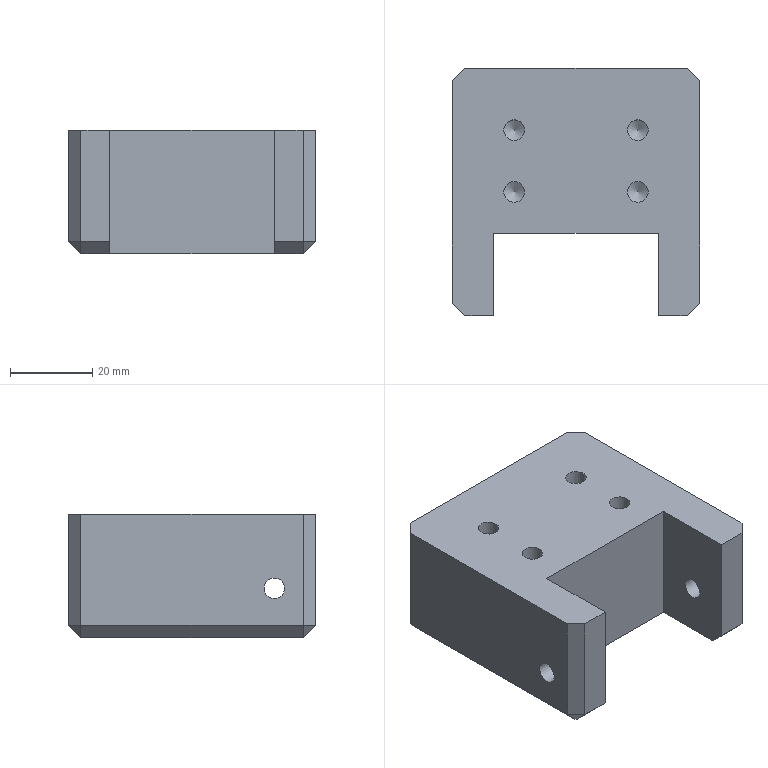Part | NX | features 5003_206_Bracket 2 | 1 solid | 33 faces | box 60 x 60 x 30 mm | volume 81572 mm3 | plane 23 | cylinder 6 | cone 4 | commonest cylinder face diameters 5 x6
STEP:
#1=CARTESIAN_POINT('',(18.525,-182.,-202.));
#2=VERTEX_POINT('',#1);
#3=CARTESIAN_POINT('',(25.525,-182.,-202.));
#4=VERTEX_POINT('',#3);
#5=CARTESIAN_POINT('',(28.525,-182.,-202.));
#6=DIRECTION('',(1.,0.,0.));
#7=VECTOR('',#6,1000.);
#8=LINE('',#5,#7);
#9=EDGE_CURVE('',#2,#4,#8,.T.);
#10=ORIENTED_EDGE('',*,*,#9,.F.);
#11=CARTESIAN_POINT('',(18.525,-182.,-229.));
#12=VERTEX_POINT('',#11);
#13=CARTESIAN_POINT('',(18.525,-182.,-201.999));
#14=DIRECTION('',(0.,0.,-1.));
#15=VECTOR('',#14,1000.);
#16=LINE('',#13,#15);
#17=EDGE_CURVE('',#2,#12,#16,.T.);
#18=ORIENTED_EDGE('',*,*,#17,.T.);
#19=CARTESIAN_POINT('',(25.525,-182.,-229.));
#20=VERTEX_POINT('',#19);
#21=CARTESIAN_POINT('',(28.525,-182.,-229.));
#22=DIRECTION('',(1.,0.,0.));
#23=VECTOR('',#22,1000.);
#24=LINE('',#21,#23);
#25=EDGE_CURVE('',#12,#20,#24,.T.);
#26=ORIENTED_EDGE('',*,*,#25,.T.);
#27=CARTESIAN_POINT('',(25.525,-182.,-202.));
#28=DIRECTION('',(0.,0.,1.));
#29=VECTOR('',#28,1000.);
#30=LINE('',#27,#29);
#31=EDGE_CURVE('',#20,#4,#30,.T.);
#32=ORIENTED_EDGE('',*,*,#31,.T.);
#33=EDGE_LOOP('',(#10,#18,#26,#32));
#34=FACE_BOUND('',#33,.T.);
#35=CARTESIAN_POINT('',(28.525,-182.,-202.));
#36=DIRECTION('',(0.,1.,0.));
#37=DIRECTION('',(-1.,0.,0.));
#38=AXIS2_PLACEMENT_3D('',#35,#36,#37);
#39=PLANE('',#38);
#40=ADVANCED_FACE('',(#34),#39,.F.);
#41=CARTESIAN_POINT('',(18.525,-169.5,-220.));
#42=VERTEX_POINT('',#41);
#43=CARTESIAN_POINT('',(18.525,-172.,-220.));
#44=DIRECTION('',(1.,0.,0.));
#45=DIRECTION('',(0.,1.,0.));
#46=AXIS2_PLACEMENT_3D('',#43,#44,#45);
#47=CIRCLE('',#46,2.5);
#48=EDGE_CURVE('',#42,#42,#47,.T.);
#49=ORIENTED_EDGE('',*,*,#48,.F.);
#50=EDGE_LOOP('',(#49));
#51=FACE_BOUND('',#50,.T.);
#52=CARTESIAN_POINT('',(28.525,-169.5,-220.));
#53=VERTEX_POINT('',#52);
#54=CARTESIAN_POINT('',(28.525,-172.,-220.));
#55=DIRECTION('',(1.,0.,0.));
#56=DIRECTION('',(0.,1.,0.));
#57=AXIS2_PLACEMENT_3D('',#54,#55,#56);
#58=CIRCLE('',#57,2.5);
#59=EDGE_CURVE('',#53,#53,#58,.T.);
#60=ORIENTED_EDGE('',*,*,#59,.T.);
#61=EDGE_LOOP('',(#60));
#62=FACE_BOUND('',#61,.T.);
#63=CARTESIAN_POINT('',(28.525,-172.,-220.));
#64=DIRECTION('',(1.,0.,0.));
#65=DIRECTION('',(0.,1.,0.));
#66=AXIS2_PLACEMENT_3D('',#63,#64,#65);
#67=CYLINDRICAL_SURFACE('',#66,2.5);
#68=ADVANCED_FACE('',(#51,#62),#67,.F.);
#69=CARTESIAN_POINT('',(18.525,-179.,-232.));
#70=VERTEX_POINT('',#69);
#71=CARTESIAN_POINT('',(18.525,-185.5,-225.5));
#72=DIRECTION('',(0.,-0.7071,0.7071));
#73=VECTOR('',#72,1000.);
#74=LINE('',#71,#73);
#75=EDGE_CURVE('',#12,#70,#74,.F.);
#76=ORIENTED_EDGE('',*,*,#75,.T.);
#77=CARTESIAN_POINT('',(25.525,-179.,-232.));
#78=VERTEX_POINT('',#77);
#79=CARTESIAN_POINT('',(28.525,-179.,-232.));
#80=DIRECTION('',(-1.,0.,0.));
#81=VECTOR('',#80,1000.);
#82=LINE('',#79,#81);
#83=EDGE_CURVE('',#78,#70,#82,.T.);
#84=ORIENTED_EDGE('',*,*,#83,.F.);
#85=CARTESIAN_POINT('',(25.525,-182.,-229.));
#86=DIRECTION('',(0.,-0.7071,0.7071));
#87=VECTOR('',#86,1000.);
#88=LINE('',#85,#87);
#89=EDGE_CURVE('',#20,#78,#88,.F.);
#90=ORIENTED_EDGE('',*,*,#89,.F.);
#91=ORIENTED_EDGE('',*,*,#25,.F.);
#92=EDGE_LOOP('',(#76,#84,#90,#91));
#93=FACE_BOUND('',#92,.T.);
#94=CARTESIAN_POINT('',(28.525,-182.,-229.));
#95=DIRECTION('',(0.,0.7071,0.7071));
#96=DIRECTION('',(1.,0.,0.));
#97=AXIS2_PLACEMENT_3D('',#94,#95,#96);
#98=PLANE('',#97);
#99=ADVANCED_FACE('',(#93),#98,.F.);
#100=ORIENTED_EDGE('',*,*,#59,.F.);
#101=EDGE_LOOP('',(#100));
#102=FACE_BOUND('',#101,.T.);
#103=CARTESIAN_POINT('',(28.525,-179.,-202.));
#104=VERTEX_POINT('',#103);
#105=CARTESIAN_POINT('',(28.525,-125.,-202.));
#106=VERTEX_POINT('',#105);
#107=CARTESIAN_POINT('',(28.525,-182.,-202.));
#108=DIRECTION('',(0.,1.,0.));
#109=VECTOR('',#108,1000.);
#110=LINE('',#107,#109);
#111=EDGE_CURVE('',#104,#106,#110,.T.);
#112=ORIENTED_EDGE('',*,*,#111,.F.);
#113=CARTESIAN_POINT('',(28.525,-179.,-229.));
#114=VERTEX_POINT('',#113);
#115=CARTESIAN_POINT('',(28.525,-179.,-202.));
#116=DIRECTION('',(0.,0.,-1.));
#117=VECTOR('',#116,1000.);
#118=LINE('',#115,#117);
#119=EDGE_CURVE('',#104,#114,#118,.T.);
#120=ORIENTED_EDGE('',*,*,#119,.T.);
#121=CARTESIAN_POINT('',(28.525,-125.,-229.));
#122=VERTEX_POINT('',#121);
#123=CARTESIAN_POINT('',(28.525,-182.,-229.));
#124=DIRECTION('',(0.,1.,0.));
#125=VECTOR('',#124,1000.);
#126=LINE('',#123,#125);
#127=EDGE_CURVE('',#114,#122,#126,.T.);
#128=ORIENTED_EDGE('',*,*,#127,.T.);
#129=CARTESIAN_POINT('',(28.525,-125.,-202.));
#130=DIRECTION('',(0.,0.,1.));
#131=VECTOR('',#130,1000.);
#132=LINE('',#129,#131);
#133=EDGE_CURVE('',#122,#106,#132,.T.);
#134=ORIENTED_EDGE('',*,*,#133,.T.);
#135=EDGE_LOOP('',(#112,#120,#128,#134));
#136=FACE_BOUND('',#135,.T.);
#137=CARTESIAN_POINT('',(28.525,-182.,-202.));
#138=DIRECTION('',(-1.,0.,0.));
#139=DIRECTION('',(0.,-1.,0.));
#140=AXIS2_PLACEMENT_3D('',#137,#138,#139);
#141=PLANE('',#140);
#142=ADVANCED_FACE('',(#102,#136),#141,.F.);
#143=CARTESIAN_POINT('',(25.525,-122.,-229.));
#144=VERTEX_POINT('',#143);
#145=CARTESIAN_POINT('',(-28.475,-122.,-229.));
#146=VERTEX_POINT('',#145);
#147=CARTESIAN_POINT('',(28.525,-122.,-229.));
#148=DIRECTION('',(-1.,0.,0.));
#149=VECTOR('',#148,1000.);
#150=LINE('',#147,#149);
#151=EDGE_CURVE('',#144,#146,#150,.T.);
#152=ORIENTED_EDGE('',*,*,#151,.T.);
#153=CARTESIAN_POINT('',(-28.475,-122.,-202.));
#154=VERTEX_POINT('',#153);
#155=CARTESIAN_POINT('',(-28.475,-122.,-202.));
#156=DIRECTION('',(0.,0.,1.));
#157=VECTOR('',#156,1000.);
#158=LINE('',#155,#157);
#159=EDGE_CURVE('',#146,#154,#158,.T.);
#160=ORIENTED_EDGE('',*,*,#159,.T.);
#161=CARTESIAN_POINT('',(25.525,-122.,-202.));
#162=VERTEX_POINT('',#161);
#163=CARTESIAN_POINT('',(28.525,-122.,-202.));
#164=DIRECTION('',(-1.,0.,0.));
#165=VECTOR('',#164,1000.);
#166=LINE('',#163,#165);
#167=EDGE_CURVE('',#162,#154,#166,.T.);
#168=ORIENTED_EDGE('',*,*,#167,.F.);
#169=CARTESIAN_POINT('',(25.525,-122.,-202.));
#170=DIRECTION('',(0.,0.,-1.));
#171=VECTOR('',#170,1000.);
#172=LINE('',#169,#171);
#173=EDGE_CURVE('',#162,#144,#172,.T.);
#174=ORIENTED_EDGE('',*,*,#173,.T.);
#175=EDGE_LOOP('',(#152,#160,#168,#174));
#176=FACE_BOUND('',#175,.T.);
#177=CARTESIAN_POINT('',(28.525,-122.,-202.));
#178=DIRECTION('',(0.,-1.,0.));
#179=DIRECTION('',(1.,0.,0.));
#180=AXIS2_PLACEMENT_3D('',#177,#178,#179);
#181=PLANE('',#180);
#182=ADVANCED_FACE('',(#176),#181,.F.);
#183=CARTESIAN_POINT('',(-31.475,-169.5,-220.));
#184=VERTEX_POINT('',#183);
#185=CARTESIAN_POINT('',(-31.475,-172.,-220.));
#186=DIRECTION('',(1.,0.,0.));
#187=DIRECTION('',(0.,1.,0.));
#188=AXIS2_PLACEMENT_3D('',#185,#186,#187);
#189=CIRCLE('',#188,2.5);
#190=EDGE_CURVE('',#184,#184,#189,.T.);
#191=ORIENTED_EDGE('',*,*,#190,.T.);
#192=EDGE_LOOP('',(#191));
#193=FACE_BOUND('',#192,.T.);
#194=CARTESIAN_POINT('',(-31.475,-125.,-202.));
#195=VERTEX_POINT('',#194);
#196=CARTESIAN_POINT('',(-31.475,-179.,-202.));
#197=VERTEX_POINT('',#196);
#198=CARTESIAN_POINT('',(-31.475,-182.,-202.));
#199=DIRECTION('',(0.,-1.,0.));
#200=VECTOR('',#199,1000.);
#201=LINE('',#198,#200);
#202=EDGE_CURVE('',#195,#197,#201,.T.);
#203=ORIENTED_EDGE('',*,*,#202,.F.);
#204=CARTESIAN_POINT('',(-31.475,-125.,-229.));
#205=VERTEX_POINT('',#204);
#206=CARTESIAN_POINT('',(-31.475,-125.,-202.));
#207=DIRECTION('',(0.,0.,-1.));
#208=VECTOR('',#207,1000.);
#209=LINE('',#206,#208);
#210=EDGE_CURVE('',#195,#205,#209,.T.);
#211=ORIENTED_EDGE('',*,*,#210,.T.);
#212=CARTESIAN_POINT('',(-31.475,-179.,-229.));
#213=VERTEX_POINT('',#212);
#214=CARTESIAN_POINT('',(-31.475,-182.,-229.));
#215=DIRECTION('',(0.,-1.,0.));
#216=VECTOR('',#215,1000.);
#217=LINE('',#214,#216);
#218=EDGE_CURVE('',#205,#213,#217,.T.);
#219=ORIENTED_EDGE('',*,*,#218,.T.);
#220=CARTESIAN_POINT('',(-31.475,-179.,-202.));
#221=DIRECTION('',(0.,0.,1.));
#222=VECTOR('',#221,1000.);
#223=LINE('',#220,#222);
#224=EDGE_CURVE('',#213,#197,#223,.T.);
#225=ORIENTED_EDGE('',*,*,#224,.T.);
#226=EDGE_LOOP('',(#203,#211,#219,#225));
#227=FACE_BOUND('',#226,.T.);
#228=CARTESIAN_POINT('',(-31.475,-182.,-202.));
#229=DIRECTION('',(1.,0.,0.));
#230=DIRECTION('',(0.,1.,0.));
#231=AXIS2_PLACEMENT_3D('',#228,#229,#230);
#232=PLANE('',#231);
#233=ADVANCED_FACE('',(#193,#227),#232,.F.);
#234=CARTESIAN_POINT('',(-28.475,-182.,-229.));
#235=VERTEX_POINT('',#234);
#236=CARTESIAN_POINT('',(-21.475,-182.,-229.));
#237=VERTEX_POINT('',#236);
#238=CARTESIAN_POINT('',(28.525,-182.,-229.));
#239=DIRECTION('',(1.,0.,0.));
#240=VECTOR('',#239,1000.);
#241=LINE('',#238,#240);
#242=EDGE_CURVE('',#235,#237,#241,.T.);
#243=ORIENTED_EDGE('',*,*,#242,.T.);
#244=CARTESIAN_POINT('',(-21.475,-182.,-202.));
#245=VERTEX_POINT('',#244);
#246=CARTESIAN_POINT('',(-21.475,-182.,-201.999));
#247=DIRECTION('',(0.,0.,-1.));
#248=VECTOR('',#247,1000.);
#249=LINE('',#246,#248);
#250=EDGE_CURVE('',#245,#237,#249,.T.);
#251=ORIENTED_EDGE('',*,*,#250,.F.);
#252=CARTESIAN_POINT('',(-28.475,-182.,-202.));
#253=VERTEX_POINT('',#252);
#254=CARTESIAN_POINT('',(28.525,-182.,-202.));
#255=DIRECTION('',(1.,0.,0.));
#256=VECTOR('',#255,1000.);
#257=LINE('',#254,#256);
#258=EDGE_CURVE('',#253,#245,#257,.T.);
#259=ORIENTED_EDGE('',*,*,#258,.F.);
#260=CARTESIAN_POINT('',(-28.475,-182.,-202.));
#261=DIRECTION('',(0.,0.,-1.));
#262=VECTOR('',#261,1000.);
#263=LINE('',#260,#262);
#264=EDGE_CURVE('',#253,#235,#263,.T.);
#265=ORIENTED_EDGE('',*,*,#264,.T.);
#266=EDGE_LOOP('',(#243,#251,#259,#265));
#267=FACE_BOUND('',#266,.T.);
#268=CARTESIAN_POINT('',(28.525,-182.,-202.));
#269=DIRECTION('',(0.,1.,0.));
#270=DIRECTION('',(-1.,0.,0.));
#271=AXIS2_PLACEMENT_3D('',#268,#269,#270);
#272=PLANE('',#271);
#273=ADVANCED_FACE('',(#267),#272,.F.);
#274=CARTESIAN_POINT('',(18.525,-162.,-202.));
#275=VERTEX_POINT('',#274);
#276=CARTESIAN_POINT('',(18.525,-162.,-202.));
#277=DIRECTION('',(0.,-1.,0.));
#278=VECTOR('',#277,1000.);
#279=LINE('',#276,#278);
#280=EDGE_CURVE('',#275,#2,#279,.T.);
#281=ORIENTED_EDGE('',*,*,#280,.T.);
#282=ORIENTED_EDGE('',*,*,#9,.T.);
#283=CARTESIAN_POINT('',(27.025,-180.5,-202.));
#284=DIRECTION('',(-0.7071,-0.7071,0.));
#285=VECTOR('',#284,1000.);
#286=LINE('',#283,#285);
#287=EDGE_CURVE('',#4,#104,#286,.F.);
#288=ORIENTED_EDGE('',*,*,#287,.T.);
#289=ORIENTED_EDGE('',*,*,#111,.T.);
#290=CARTESIAN_POINT('',(57.025,-153.5,-202.));
#291=DIRECTION('',(0.7071,-0.7071,0.));
#292=VECTOR('',#291,1000.);
#293=LINE('',#290,#292);
#294=EDGE_CURVE('',#106,#162,#293,.F.);
#295=ORIENTED_EDGE('',*,*,#294,.T.);
#296=ORIENTED_EDGE('',*,*,#167,.T.);
#297=CARTESIAN_POINT('',(-29.975,-123.5,-202.));
#298=DIRECTION('',(0.7071,0.7071,0.));
#299=VECTOR('',#298,1000.);
#300=LINE('',#297,#299);
#301=EDGE_CURVE('',#154,#195,#300,.F.);
#302=ORIENTED_EDGE('',*,*,#301,.T.);
#303=ORIENTED_EDGE('',*,*,#202,.T.);
#304=CARTESIAN_POINT('',(0.025,-210.5,-202.));
#305=DIRECTION('',(-0.7071,0.7071,0.));
#306=VECTOR('',#305,1000.);
#307=LINE('',#304,#306);
#308=EDGE_CURVE('',#197,#253,#307,.F.);
#309=ORIENTED_EDGE('',*,*,#308,.T.);
#310=ORIENTED_EDGE('',*,*,#258,.T.);
#311=CARTESIAN_POINT('',(-21.475,-162.,-202.));
#312=VERTEX_POINT('',#311);
#313=CARTESIAN_POINT('',(-21.475,-162.,-202.));
#314=DIRECTION('',(0.,1.,0.));
#315=VECTOR('',#314,1000.);
#316=LINE('',#313,#315);
#317=EDGE_CURVE('',#245,#312,#316,.T.);
#318=ORIENTED_EDGE('',*,*,#317,.T.);
#319=CARTESIAN_POINT('',(18.525,-162.,-202.));
#320=DIRECTION('',(1.,0.,0.));
#321=VECTOR('',#320,1000.);
#322=LINE('',#319,#321);
#323=EDGE_CURVE('',#312,#275,#322,.T.);
#324=ORIENTED_EDGE('',*,*,#323,.T.);
#325=EDGE_LOOP('',(#281,#282,#288,#289,#295,#296,#302,#303,#309,#310,#318,#324));
#326=FACE_BOUND('',#325,.T.);
#327=CARTESIAN_POINT('',(-16.475,-149.5,-202.));
#328=VERTEX_POINT('',#327);
#329=CARTESIAN_POINT('',(-16.475,-152.,-202.));
#330=DIRECTION('',(0.,0.,1.));
#331=DIRECTION('',(0.,1.,0.));
#332=AXIS2_PLACEMENT_3D('',#329,#330,#331);
#333=CIRCLE('',#332,2.5);
#334=EDGE_CURVE('',#328,#328,#333,.T.);
#335=ORIENTED_EDGE('',*,*,#334,.F.);
#336=EDGE_LOOP('',(#335));
#337=FACE_BOUND('',#336,.T.);
#338=CARTESIAN_POINT('',(13.525,-134.5,-202.));
#339=VERTEX_POINT('',#338);
#340=CARTESIAN_POINT('',(13.525,-137.,-202.));
#341=DIRECTION('',(0.,0.,1.));
#342=DIRECTION('',(0.,1.,0.));
#343=AXIS2_PLACEMENT_3D('',#340,#341,#342);
#344=CIRCLE('',#343,2.5);
#345=EDGE_CURVE('',#339,#339,#344,.T.);
#346=ORIENTED_EDGE('',*,*,#345,.F.);
#347=EDGE_LOOP('',(#346));
#348=FACE_BOUND('',#347,.T.);
#349=CARTESIAN_POINT('',(-16.475,-134.5,-202.));
#350=VERTEX_POINT('',#349);
#351=CARTESIAN_POINT('',(-16.475,-137.,-202.));
#352=DIRECTION('',(0.,0.,1.));
#353=DIRECTION('',(0.,1.,0.));
#354=AXIS2_PLACEMENT_3D('',#351,#352,#353);
#355=CIRCLE('',#354,2.5);
#356=EDGE_CURVE('',#350,#350,#355,.T.);
#357=ORIENTED_EDGE('',*,*,#356,.F.);
#358=EDGE_LOOP('',(#357));
#359=FACE_BOUND('',#358,.T.);
#360=CARTESIAN_POINT('',(13.525,-149.5,-202.));
#361=VERTEX_POINT('',#360);
#362=CARTESIAN_POINT('',(13.525,-152.,-202.));
#363=DIRECTION('',(0.,0.,1.));
#364=DIRECTION('',(0.,1.,0.));
#365=AXIS2_PLACEMENT_3D('',#362,#363,#364);
#366=CIRCLE('',#365,2.5);
#367=EDGE_CURVE('',#361,#361,#366,.T.);
#368=ORIENTED_EDGE('',*,*,#367,.F.);
#369=EDGE_LOOP('',(#368));
#370=FACE_BOUND('',#369,.T.);
#371=CARTESIAN_POINT('',(28.525,-182.,-202.));
#372=DIRECTION('',(0.,0.,1.));
#373=DIRECTION('',(0.,1.,0.));
#374=AXIS2_PLACEMENT_3D('',#371,#372,#373);
#375=PLANE('',#374);
#376=ADVANCED_FACE('',(#326,#337,#348,#359,#370),#375,.T.);
#377=ORIENTED_EDGE('',*,*,#83,.T.);
#378=CARTESIAN_POINT('',(18.525,-162.,-232.));
#379=VERTEX_POINT('',#378);
#380=CARTESIAN_POINT('',(18.525,-162.,-232.));
#381=DIRECTION('',(0.,-1.,0.));
#382=VECTOR('',#381,1000.);
#383=LINE('',#380,#382);
#384=EDGE_CURVE('',#379,#70,#383,.T.);
#385=ORIENTED_EDGE('',*,*,#384,.F.);
#386=CARTESIAN_POINT('',(-21.475,-162.,-232.));
#387=VERTEX_POINT('',#386);
#388=CARTESIAN_POINT('',(18.525,-162.,-232.));
#389=DIRECTION('',(1.,0.,0.));
#390=VECTOR('',#389,1000.);
#391=LINE('',#388,#390);
#392=EDGE_CURVE('',#387,#379,#391,.T.);
#393=ORIENTED_EDGE('',*,*,#392,.F.);
#394=CARTESIAN_POINT('',(-21.475,-179.,-232.));
#395=VERTEX_POINT('',#394);
#396=CARTESIAN_POINT('',(-21.475,-162.,-232.));
#397=DIRECTION('',(0.,1.,0.));
#398=VECTOR('',#397,1000.);
#399=LINE('',#396,#398);
#400=EDGE_CURVE('',#395,#387,#399,.T.);
#401=ORIENTED_EDGE('',*,*,#400,.F.);
#402=CARTESIAN_POINT('',(-28.475,-179.,-232.));
#403=VERTEX_POINT('',#402);
#404=CARTESIAN_POINT('',(28.525,-179.,-232.));
#405=DIRECTION('',(-1.,0.,0.));
#406=VECTOR('',#405,1000.);
#407=LINE('',#404,#406);
#408=EDGE_CURVE('',#395,#403,#407,.T.);
#409=ORIENTED_EDGE('',*,*,#408,.T.);
#410=CARTESIAN_POINT('',(-28.475,-125.,-232.));
#411=VERTEX_POINT('',#410);
#412=CARTESIAN_POINT('',(-28.475,-182.,-232.));
#413=DIRECTION('',(0.,1.,0.));
#414=VECTOR('',#413,1000.);
#415=LINE('',#412,#414);
#416=EDGE_CURVE('',#403,#411,#415,.T.);
#417=ORIENTED_EDGE('',*,*,#416,.T.);
#418=CARTESIAN_POINT('',(25.525,-125.,-232.));
#419=VERTEX_POINT('',#418);
#420=CARTESIAN_POINT('',(28.525,-125.,-232.));
#421=DIRECTION('',(1.,0.,0.));
#422=VECTOR('',#421,1000.);
#423=LINE('',#420,#422);
#424=EDGE_CURVE('',#411,#419,#423,.T.);
#425=ORIENTED_EDGE('',*,*,#424,.T.);
#426=CARTESIAN_POINT('',(25.525,-182.,-232.));
#427=DIRECTION('',(0.,-1.,0.));
#428=VECTOR('',#427,1000.);
#429=LINE('',#426,#428);
#430=EDGE_CURVE('',#419,#78,#429,.T.);
#431=ORIENTED_EDGE('',*,*,#430,.T.);
#432=EDGE_LOOP('',(#377,#385,#393,#401,#409,#417,#425,#431));
#433=FACE_BOUND('',#432,.T.);
#434=CARTESIAN_POINT('',(28.525,-182.,-232.));
#435=DIRECTION('',(0.,0.,1.));
#436=DIRECTION('',(0.,1.,0.));
#437=AXIS2_PLACEMENT_3D('',#434,#435,#436);
#438=PLANE('',#437);
#439=ADVANCED_FACE('',(#433),#438,.F.);
#440=CARTESIAN_POINT('',(-21.475,-174.5,-220.));
#441=VERTEX_POINT('',#440);
#442=CARTESIAN_POINT('',(-21.475,-172.,-220.));
#443=DIRECTION('',(-1.,0.,0.));
#444=DIRECTION('',(0.,-1.,0.));
#445=AXIS2_PLACEMENT_3D('',#442,#443,#444);
#446=CIRCLE('',#445,2.5);
#447=EDGE_CURVE('',#441,#441,#446,.T.);
#448=ORIENTED_EDGE('',*,*,#447,.F.);
#449=EDGE_LOOP('',(#448));
#450=FACE_BOUND('',#449,.T.);
#451=ORIENTED_EDGE('',*,*,#190,.F.);
#452=EDGE_LOOP('',(#451));
#453=FACE_BOUND('',#452,.T.);
#454=CARTESIAN_POINT('',(28.525,-172.,-220.));
#455=DIRECTION('',(1.,0.,0.));
#456=DIRECTION('',(0.,1.,0.));
#457=AXIS2_PLACEMENT_3D('',#454,#455,#456);
#458=CYLINDRICAL_SURFACE('',#457,2.5);
#459=ADVANCED_FACE('',(#450,#453),#458,.F.);
#460=CARTESIAN_POINT('',(13.525,-152.,-211.502));
#461=VERTEX_POINT('',#460);
#462=VERTEX_LOOP('',#461);
#463=FACE_BOUND('',#462,.T.);
#464=CARTESIAN_POINT('',(13.525,-149.5,-210.));
#465=VERTEX_POINT('',#464);
#466=CARTESIAN_POINT('',(13.525,-152.,-210.));
#467=DIRECTION('',(0.,0.,1.));
#468=DIRECTION('',(0.,1.,0.));
#469=AXIS2_PLACEMENT_3D('',#466,#467,#468);
#470=CIRCLE('',#469,2.5);
#471=EDGE_CURVE('',#465,#465,#470,.T.);
#472=ORIENTED_EDGE('',*,*,#471,.T.);
#473=EDGE_LOOP('',(#472));
#474=FACE_BOUND('',#473,.T.);
#475=CARTESIAN_POINT('',(13.525,-152.,-210.));
#476=DIRECTION('',(0.,0.,1.));
#477=DIRECTION('',(0.,1.,0.));
#478=AXIS2_PLACEMENT_3D('',#475,#476,#477);
#479=CONICAL_SURFACE('',#478,2.5,1.03);
#480=ADVANCED_FACE('',(#463,#474),#479,.F.);
#481=ORIENTED_EDGE('',*,*,#471,.F.);
#482=EDGE_LOOP('',(#481));
#483=FACE_BOUND('',#482,.T.);
#484=ORIENTED_EDGE('',*,*,#367,.T.);
#485=EDGE_LOOP('',(#484));
#486=FACE_BOUND('',#485,.T.);
#487=CARTESIAN_POINT('',(13.525,-152.,-202.));
#488=DIRECTION('',(0.,0.,1.));
#489=DIRECTION('',(0.,1.,0.));
#490=AXIS2_PLACEMENT_3D('',#487,#488,#489);
#491=CYLINDRICAL_SURFACE('',#490,2.5);
#492=ADVANCED_FACE('',(#483,#486),#491,.F.);
#493=CARTESIAN_POINT('',(-16.475,-137.,-211.502));
#494=VERTEX_POINT('',#493);
#495=VERTEX_LOOP('',#494);
#496=FACE_BOUND('',#495,.T.);
#497=CARTESIAN_POINT('',(-16.475,-134.5,-210.));
#498=VERTEX_POINT('',#497);
#499=CARTESIAN_POINT('',(-16.475,-137.,-210.));
#500=DIRECTION('',(0.,0.,1.));
#501=DIRECTION('',(0.,1.,0.));
#502=AXIS2_PLACEMENT_3D('',#499,#500,#501);
#503=CIRCLE('',#502,2.5);
#504=EDGE_CURVE('',#498,#498,#503,.T.);
#505=ORIENTED_EDGE('',*,*,#504,.T.);
#506=EDGE_LOOP('',(#505));
#507=FACE_BOUND('',#506,.T.);
#508=CARTESIAN_POINT('',(-16.475,-137.,-210.));
#509=DIRECTION('',(0.,0.,1.));
#510=DIRECTION('',(0.,1.,0.));
#511=AXIS2_PLACEMENT_3D('',#508,#509,#510);
#512=CONICAL_SURFACE('',#511,2.5,1.03);
#513=ADVANCED_FACE('',(#496,#507),#512,.F.);
#514=ORIENTED_EDGE('',*,*,#504,.F.);
#515=EDGE_LOOP('',(#514));
#516=FACE_BOUND('',#515,.T.);
#517=ORIENTED_EDGE('',*,*,#356,.T.);
#518=EDGE_LOOP('',(#517));
#519=FACE_BOUND('',#518,.T.);
#520=CARTESIAN_POINT('',(-16.475,-137.,-202.));
#521=DIRECTION('',(0.,0.,1.));
#522=DIRECTION('',(0.,1.,0.));
#523=AXIS2_PLACEMENT_3D('',#520,#521,#522);
#524=CYLINDRICAL_SURFACE('',#523,2.5);
#525=ADVANCED_FACE('',(#516,#519),#524,.F.);
#526=CARTESIAN_POINT('',(13.525,-137.,-211.502));
#527=VERTEX_POINT('',#526);
#528=VERTEX_LOOP('',#527);
#529=FACE_BOUND('',#528,.T.);
#530=CARTESIAN_POINT('',(13.525,-134.5,-210.));
#531=VERTEX_POINT('',#530);
#532=CARTESIAN_POINT('',(13.525,-137.,-210.));
#533=DIRECTION('',(0.,0.,1.));
#534=DIRECTION('',(0.,1.,0.));
#535=AXIS2_PLACEMENT_3D('',#532,#533,#534);
#536=CIRCLE('',#535,2.5);
#537=EDGE_CURVE('',#531,#531,#536,.T.);
#538=ORIENTED_EDGE('',*,*,#537,.T.);
#539=EDGE_LOOP('',(#538));
#540=FACE_BOUND('',#539,.T.);
#541=CARTESIAN_POINT('',(13.525,-137.,-210.));
#542=DIRECTION('',(0.,0.,1.));
#543=DIRECTION('',(0.,1.,0.));
#544=AXIS2_PLACEMENT_3D('',#541,#542,#543);
#545=CONICAL_SURFACE('',#544,2.5,1.03);
#546=ADVANCED_FACE('',(#529,#540),#545,.F.);
#547=ORIENTED_EDGE('',*,*,#537,.F.);
#548=EDGE_LOOP('',(#547));
#549=FACE_BOUND('',#548,.T.);
#550=ORIENTED_EDGE('',*,*,#345,.T.);
#551=EDGE_LOOP('',(#550));
#552=FACE_BOUND('',#551,.T.);
#553=CARTESIAN_POINT('',(13.525,-137.,-202.));
#554=DIRECTION('',(0.,0.,1.));
#555=DIRECTION('',(0.,1.,0.));
#556=AXIS2_PLACEMENT_3D('',#553,#554,#555);
#557=CYLINDRICAL_SURFACE('',#556,2.5);
#558=ADVANCED_FACE('',(#549,#552),#557,.F.);
#559=CARTESIAN_POINT('',(-16.475,-152.,-211.502));
#560=VERTEX_POINT('',#559);
#561=VERTEX_LOOP('',#560);
#562=FACE_BOUND('',#561,.T.);
#563=CARTESIAN_POINT('',(-16.475,-149.5,-210.));
#564=VERTEX_POINT('',#563);
#565=CARTESIAN_POINT('',(-16.475,-152.,-210.));
#566=DIRECTION('',(0.,0.,1.));
#567=DIRECTION('',(0.,1.,0.));
#568=AXIS2_PLACEMENT_3D('',#565,#566,#567);
#569=CIRCLE('',#568,2.5);
#570=EDGE_CURVE('',#564,#564,#569,.T.);
#571=ORIENTED_EDGE('',*,*,#570,.T.);
#572=EDGE_LOOP('',(#571));
#573=FACE_BOUND('',#572,.T.);
#574=CARTESIAN_POINT('',(-16.475,-152.,-210.));
#575=DIRECTION('',(0.,0.,1.));
#576=DIRECTION('',(0.,1.,0.));
#577=AXIS2_PLACEMENT_3D('',#574,#575,#576);
#578=CONICAL_SURFACE('',#577,2.5,1.03);
#579=ADVANCED_FACE('',(#562,#573),#578,.F.);
#580=ORIENTED_EDGE('',*,*,#570,.F.);
#581=EDGE_LOOP('',(#580));
#582=FACE_BOUND('',#581,.T.);
#583=ORIENTED_EDGE('',*,*,#334,.T.);
#584=EDGE_LOOP('',(#583));
#585=FACE_BOUND('',#584,.T.);
#586=CARTESIAN_POINT('',(-16.475,-152.,-202.));
#587=DIRECTION('',(0.,0.,1.));
#588=DIRECTION('',(0.,1.,0.));
#589=AXIS2_PLACEMENT_3D('',#586,#587,#588);
#590=CYLINDRICAL_SURFACE('',#589,2.5);
#591=ADVANCED_FACE('',(#582,#585),#590,.F.);
#592=ORIENTED_EDGE('',*,*,#287,.F.);
#593=ORIENTED_EDGE('',*,*,#31,.F.);
#594=CARTESIAN_POINT('',(25.525,-182.,-229.));
#595=DIRECTION('',(0.7071,0.7071,0.));
#596=VECTOR('',#595,1000.);
#597=LINE('',#594,#596);
#598=EDGE_CURVE('',#114,#20,#597,.F.);
#599=ORIENTED_EDGE('',*,*,#598,.F.);
#600=ORIENTED_EDGE('',*,*,#119,.F.);
#601=EDGE_LOOP('',(#592,#593,#599,#600));
#602=FACE_BOUND('',#601,.T.);
#603=CARTESIAN_POINT('',(28.525,-179.,-202.));
#604=DIRECTION('',(-0.7071,0.7071,0.));
#605=DIRECTION('',(0.,0.,-1.));
#606=AXIS2_PLACEMENT_3D('',#603,#604,#605);
#607=PLANE('',#606);
#608=ADVANCED_FACE('',(#602),#607,.F.);
#609=ORIENTED_EDGE('',*,*,#308,.F.);
#610=ORIENTED_EDGE('',*,*,#224,.F.);
#611=CARTESIAN_POINT('',(-31.475,-179.,-229.));
#612=DIRECTION('',(0.7071,-0.7071,0.));
#613=VECTOR('',#612,1000.);
#614=LINE('',#611,#613);
#615=EDGE_CURVE('',#235,#213,#614,.F.);
#616=ORIENTED_EDGE('',*,*,#615,.F.);
#617=ORIENTED_EDGE('',*,*,#264,.F.);
#618=EDGE_LOOP('',(#609,#610,#616,#617));
#619=FACE_BOUND('',#618,.T.);
#620=CARTESIAN_POINT('',(-28.475,-182.,-202.));
#621=DIRECTION('',(0.7071,0.7071,0.));
#622=DIRECTION('',(0.,0.,-1.));
#623=AXIS2_PLACEMENT_3D('',#620,#621,#622);
#624=PLANE('',#623);
#625=ADVANCED_FACE('',(#619),#624,.F.);
#626=CARTESIAN_POINT('',(-21.475,-185.5,-225.5));
#627=DIRECTION('',(0.,0.7071,-0.7071));
#628=VECTOR('',#627,1000.);
#629=LINE('',#626,#628);
#630=EDGE_CURVE('',#395,#237,#629,.F.);
#631=ORIENTED_EDGE('',*,*,#630,.T.);
#632=ORIENTED_EDGE('',*,*,#242,.F.);
#633=CARTESIAN_POINT('',(-28.475,-180.5,-230.5));
#634=DIRECTION('',(0.,0.7071,-0.7071));
#635=VECTOR('',#634,1000.);
#636=LINE('',#633,#635);
#637=EDGE_CURVE('',#403,#235,#636,.F.);
#638=ORIENTED_EDGE('',*,*,#637,.F.);
#639=ORIENTED_EDGE('',*,*,#408,.F.);
#640=EDGE_LOOP('',(#631,#632,#638,#639));
#641=FACE_BOUND('',#640,.T.);
#642=CARTESIAN_POINT('',(28.525,-182.,-229.));
#643=DIRECTION('',(0.,0.7071,0.7071));
#644=DIRECTION('',(1.,0.,0.));
#645=AXIS2_PLACEMENT_3D('',#642,#643,#644);
#646=PLANE('',#645);
#647=ADVANCED_FACE('',(#641),#646,.F.);
#648=ORIENTED_EDGE('',*,*,#598,.T.);
#649=ORIENTED_EDGE('',*,*,#89,.T.);
#650=CARTESIAN_POINT('',(27.025,-179.,-230.5));
#651=DIRECTION('',(-0.7071,0.,-0.7071));
#652=VECTOR('',#651,1000.);
#653=LINE('',#650,#652);
#654=EDGE_CURVE('',#114,#78,#653,.T.);
#655=ORIENTED_EDGE('',*,*,#654,.F.);
#656=EDGE_LOOP('',(#648,#649,#655));
#657=FACE_BOUND('',#656,.T.);
#658=CARTESIAN_POINT('',(25.525,-182.,-229.));
#659=DIRECTION('',(0.5774,-0.5774,-0.5774));
#660=DIRECTION('',(-0.7071,0.,-0.7071));
#661=AXIS2_PLACEMENT_3D('',#658,#659,#660);
#662=PLANE('',#661);
#663=ADVANCED_FACE('',(#657),#662,.T.);
#664=ORIENTED_EDGE('',*,*,#637,.T.);
#665=ORIENTED_EDGE('',*,*,#615,.T.);
#666=CARTESIAN_POINT('',(-31.475,-179.,-229.));
#667=DIRECTION('',(-0.7071,0.,0.7071));
#668=VECTOR('',#667,1000.);
#669=LINE('',#666,#668);
#670=EDGE_CURVE('',#403,#213,#669,.T.);
#671=ORIENTED_EDGE('',*,*,#670,.F.);
#672=EDGE_LOOP('',(#664,#665,#671));
#673=FACE_BOUND('',#672,.T.);
#674=CARTESIAN_POINT('',(-31.475,-179.,-229.));
#675=DIRECTION('',(-0.5774,-0.5774,-0.5774));
#676=DIRECTION('',(-0.7071,0.,0.7071));
#677=AXIS2_PLACEMENT_3D('',#674,#675,#676);
#678=PLANE('',#677);
#679=ADVANCED_FACE('',(#673),#678,.T.);
#680=ORIENTED_EDGE('',*,*,#654,.T.);
#681=ORIENTED_EDGE('',*,*,#430,.F.);
#682=CARTESIAN_POINT('',(25.525,-125.,-232.));
#683=DIRECTION('',(0.7071,0.,0.7071));
#684=VECTOR('',#683,1000.);
#685=LINE('',#682,#684);
#686=EDGE_CURVE('',#122,#419,#685,.F.);
#687=ORIENTED_EDGE('',*,*,#686,.F.);
#688=ORIENTED_EDGE('',*,*,#127,.F.);
#689=EDGE_LOOP('',(#680,#681,#687,#688));
#690=FACE_BOUND('',#689,.T.);
#691=CARTESIAN_POINT('',(28.525,-182.,-229.));
#692=DIRECTION('',(-0.7071,0.,0.7071));
#693=DIRECTION('',(0.,1.,0.));
#694=AXIS2_PLACEMENT_3D('',#691,#692,#693);
#695=PLANE('',#694);
#696=ADVANCED_FACE('',(#690),#695,.F.);
#697=ORIENTED_EDGE('',*,*,#294,.F.);
#698=ORIENTED_EDGE('',*,*,#133,.F.);
#699=CARTESIAN_POINT('',(27.025,-123.5,-229.));
#700=DIRECTION('',(-0.7071,0.7071,0.));
#701=VECTOR('',#700,1000.);
#702=LINE('',#699,#701);
#703=EDGE_CURVE('',#144,#122,#702,.F.);
#704=ORIENTED_EDGE('',*,*,#703,.F.);
#705=ORIENTED_EDGE('',*,*,#173,.F.);
#706=EDGE_LOOP('',(#697,#698,#704,#705));
#707=FACE_BOUND('',#706,.T.);
#708=CARTESIAN_POINT('',(25.525,-122.,-202.));
#709=DIRECTION('',(-0.7071,-0.7071,0.));
#710=DIRECTION('',(0.,0.,-1.));
#711=AXIS2_PLACEMENT_3D('',#708,#709,#710);
#712=PLANE('',#711);
#713=ADVANCED_FACE('',(#707),#712,.F.);
#714=ORIENTED_EDGE('',*,*,#301,.F.);
#715=ORIENTED_EDGE('',*,*,#159,.F.);
#716=CARTESIAN_POINT('',(-28.475,-122.,-229.));
#717=DIRECTION('',(-0.7071,-0.7071,0.));
#718=VECTOR('',#717,1000.);
#719=LINE('',#716,#718);
#720=EDGE_CURVE('',#205,#146,#719,.F.);
#721=ORIENTED_EDGE('',*,*,#720,.F.);
#722=ORIENTED_EDGE('',*,*,#210,.F.);
#723=EDGE_LOOP('',(#714,#715,#721,#722));
#724=FACE_BOUND('',#723,.T.);
#725=CARTESIAN_POINT('',(-31.475,-125.,-202.));
#726=DIRECTION('',(0.7071,-0.7071,0.));
#727=DIRECTION('',(0.,0.,-1.));
#728=AXIS2_PLACEMENT_3D('',#725,#726,#727);
#729=PLANE('',#728);
#730=ADVANCED_FACE('',(#724),#729,.F.);
#731=ORIENTED_EDGE('',*,*,#670,.T.);
#732=ORIENTED_EDGE('',*,*,#218,.F.);
#733=CARTESIAN_POINT('',(-29.975,-125.,-230.5));
#734=DIRECTION('',(0.7071,0.,-0.7071));
#735=VECTOR('',#734,1000.);
#736=LINE('',#733,#735);
#737=EDGE_CURVE('',#411,#205,#736,.F.);
#738=ORIENTED_EDGE('',*,*,#737,.F.);
#739=ORIENTED_EDGE('',*,*,#416,.F.);
#740=EDGE_LOOP('',(#731,#732,#738,#739));
#741=FACE_BOUND('',#740,.T.);
#742=CARTESIAN_POINT('',(-31.475,-182.,-229.));
#743=DIRECTION('',(0.7071,0.,0.7071));
#744=DIRECTION('',(0.,-1.,0.));
#745=AXIS2_PLACEMENT_3D('',#742,#743,#744);
#746=PLANE('',#745);
#747=ADVANCED_FACE('',(#741),#746,.F.);
#748=ORIENTED_EDGE('',*,*,#703,.T.);
#749=ORIENTED_EDGE('',*,*,#686,.T.);
#750=CARTESIAN_POINT('',(25.525,-125.,-232.));
#751=DIRECTION('',(0.,-0.7071,-0.7071));
#752=VECTOR('',#751,1000.);
#753=LINE('',#750,#752);
#754=EDGE_CURVE('',#144,#419,#753,.T.);
#755=ORIENTED_EDGE('',*,*,#754,.F.);
#756=EDGE_LOOP('',(#748,#749,#755));
#757=FACE_BOUND('',#756,.T.);
#758=CARTESIAN_POINT('',(25.525,-125.,-232.));
#759=DIRECTION('',(0.5774,0.5774,-0.5774));
#760=DIRECTION('',(-0.7071,0.,-0.7071));
#761=AXIS2_PLACEMENT_3D('',#758,#759,#760);
#762=PLANE('',#761);
#763=ADVANCED_FACE('',(#757),#762,.T.);
#764=ORIENTED_EDGE('',*,*,#737,.T.);
#765=ORIENTED_EDGE('',*,*,#720,.T.);
#766=CARTESIAN_POINT('',(-28.475,-122.,-229.));
#767=DIRECTION('',(0.,0.7071,0.7071));
#768=VECTOR('',#767,1000.);
#769=LINE('',#766,#768);
#770=EDGE_CURVE('',#411,#146,#769,.T.);
#771=ORIENTED_EDGE('',*,*,#770,.F.);
#772=EDGE_LOOP('',(#764,#765,#771));
#773=FACE_BOUND('',#772,.T.);
#774=CARTESIAN_POINT('',(-28.475,-122.,-229.));
#775=DIRECTION('',(-0.5774,0.5774,-0.5774));
#776=DIRECTION('',(-0.7071,0.,0.7071));
#777=AXIS2_PLACEMENT_3D('',#774,#775,#776);
#778=PLANE('',#777);
#779=ADVANCED_FACE('',(#773),#778,.T.);
#780=ORIENTED_EDGE('',*,*,#754,.T.);
#781=ORIENTED_EDGE('',*,*,#424,.F.);
#782=ORIENTED_EDGE('',*,*,#770,.T.);
#783=ORIENTED_EDGE('',*,*,#151,.F.);
#784=EDGE_LOOP('',(#780,#781,#782,#783));
#785=FACE_BOUND('',#784,.T.);
#786=CARTESIAN_POINT('',(28.525,-122.,-229.));
#787=DIRECTION('',(0.,-0.7071,0.7071));
#788=DIRECTION('',(-1.,0.,0.));
#789=AXIS2_PLACEMENT_3D('',#786,#787,#788);
#790=PLANE('',#789);
#791=ADVANCED_FACE('',(#785),#790,.F.);
#792=CARTESIAN_POINT('',(18.525,-162.,-201.999));
#793=DIRECTION('',(0.,0.,-1.));
#794=VECTOR('',#793,1000.);
#795=LINE('',#792,#794);
#796=EDGE_CURVE('',#275,#379,#795,.T.);
#797=ORIENTED_EDGE('',*,*,#796,.T.);
#798=ORIENTED_EDGE('',*,*,#384,.T.);
#799=ORIENTED_EDGE('',*,*,#75,.F.);
#800=ORIENTED_EDGE('',*,*,#17,.F.);
#801=ORIENTED_EDGE('',*,*,#280,.F.);
#802=EDGE_LOOP('',(#797,#798,#799,#800,#801));
#803=FACE_BOUND('',#802,.T.);
#804=ORIENTED_EDGE('',*,*,#48,.T.);
#805=EDGE_LOOP('',(#804));
#806=FACE_BOUND('',#805,.T.);
#807=CARTESIAN_POINT('',(18.525,-162.,-201.999));
#808=DIRECTION('',(1.,0.,0.));
#809=DIRECTION('',(0.,1.,0.));
#810=AXIS2_PLACEMENT_3D('',#807,#808,#809);
#811=PLANE('',#810);
#812=ADVANCED_FACE('',(#803,#806),#811,.F.);
#813=ORIENTED_EDGE('',*,*,#250,.T.);
#814=ORIENTED_EDGE('',*,*,#630,.F.);
#815=ORIENTED_EDGE('',*,*,#400,.T.);
#816=CARTESIAN_POINT('',(-21.475,-162.,-201.999));
#817=DIRECTION('',(0.,0.,-1.));
#818=VECTOR('',#817,1000.);
#819=LINE('',#816,#818);
#820=EDGE_CURVE('',#312,#387,#819,.T.);
#821=ORIENTED_EDGE('',*,*,#820,.F.);
#822=ORIENTED_EDGE('',*,*,#317,.F.);
#823=EDGE_LOOP('',(#813,#814,#815,#821,#822));
#824=FACE_BOUND('',#823,.T.);
#825=ORIENTED_EDGE('',*,*,#447,.T.);
#826=EDGE_LOOP('',(#825));
#827=FACE_BOUND('',#826,.T.);
#828=CARTESIAN_POINT('',(-21.475,-162.,-201.999));
#829=DIRECTION('',(-1.,0.,0.));
#830=DIRECTION('',(0.,-1.,0.));
#831=AXIS2_PLACEMENT_3D('',#828,#829,#830);
#832=PLANE('',#831);
#833=ADVANCED_FACE('',(#824,#827),#832,.F.);
#834=ORIENTED_EDGE('',*,*,#820,.T.);
#835=ORIENTED_EDGE('',*,*,#392,.T.);
#836=ORIENTED_EDGE('',*,*,#796,.F.);
#837=ORIENTED_EDGE('',*,*,#323,.F.);
#838=EDGE_LOOP('',(#834,#835,#836,#837));
#839=FACE_BOUND('',#838,.T.);
#840=CARTESIAN_POINT('',(18.525,-162.,-201.999));
#841=DIRECTION('',(0.,1.,0.));
#842=DIRECTION('',(-1.,0.,0.));
#843=AXIS2_PLACEMENT_3D('',#840,#841,#842);
#844=PLANE('',#843);
#845=ADVANCED_FACE('',(#839),#844,.F.);
#846=CLOSED_SHELL('',(#40,#68,#99,#142,#182,#233,#273,#376,#439,#459,#480,#492,#513,#525,#546,#558,#579,#591,#608,#625,#647,#663,#679,#696,#713,#730,#747,#763,#779,#791,#812,#833,#845));
#847=MANIFOLD_SOLID_BREP('',#846);
#848=(LENGTH_UNIT()NAMED_UNIT(*)SI_UNIT(.MILLI.,.METRE.));
#849=UNCERTAINTY_MEASURE_WITH_UNIT(LENGTH_MEASURE(0.00001),#848,'','');
#850=(NAMED_UNIT(*)PLANE_ANGLE_UNIT()SI_UNIT($,.RADIAN.));
#851=(NAMED_UNIT(*)SI_UNIT($,.STERADIAN.)SOLID_ANGLE_UNIT());
#852=(GEOMETRIC_REPRESENTATION_CONTEXT(3)GLOBAL_UNCERTAINTY_ASSIGNED_CONTEXT((#849))GLOBAL_UNIT_ASSIGNED_CONTEXT((#848,#850,#851))REPRESENTATION_CONTEXT('',''));
#853=ADVANCED_BREP_SHAPE_REPRESENTATION('',(#847),#852);